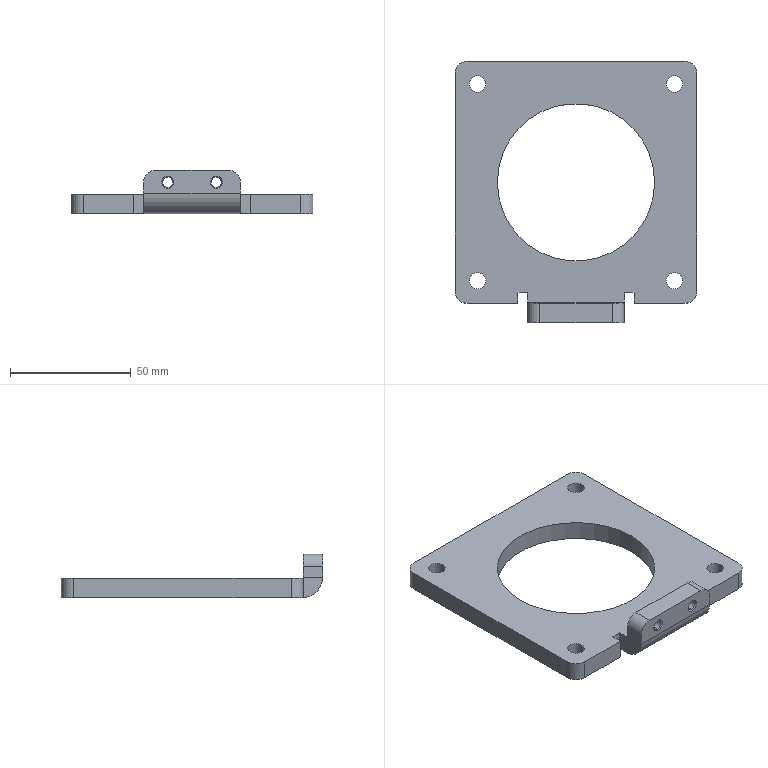Part | STEP file | 1 solid | 46 faces | box 100 x 108 x 18.001 mm | volume 56664 mm3 | cylinder 22 | plane 20 | cone 4 | commonest cylinder face diameters 6.8 x8 10 x6 4.2 x4 65 x2 1 x1 17 x1